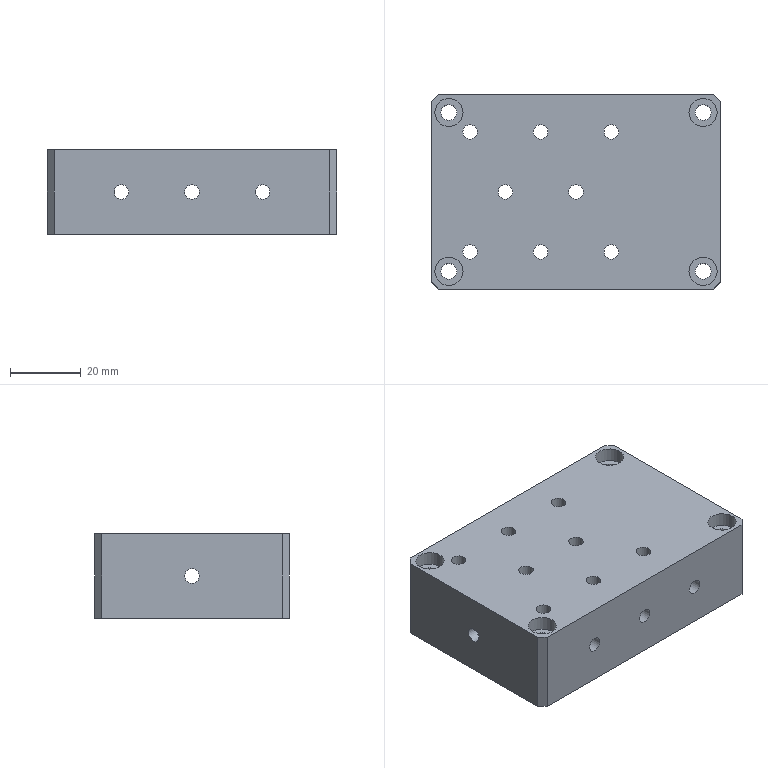Part | 1 solid | 66 faces | box 82 x 55 x 24 mm | volume 56642 mm3 | cylinder 36 | plane 29 | cone 1 | commonest cylinder face diameters 4.134 x15 4.5 x4 8 x4 12 x4 13.6 x4 16.6 x4